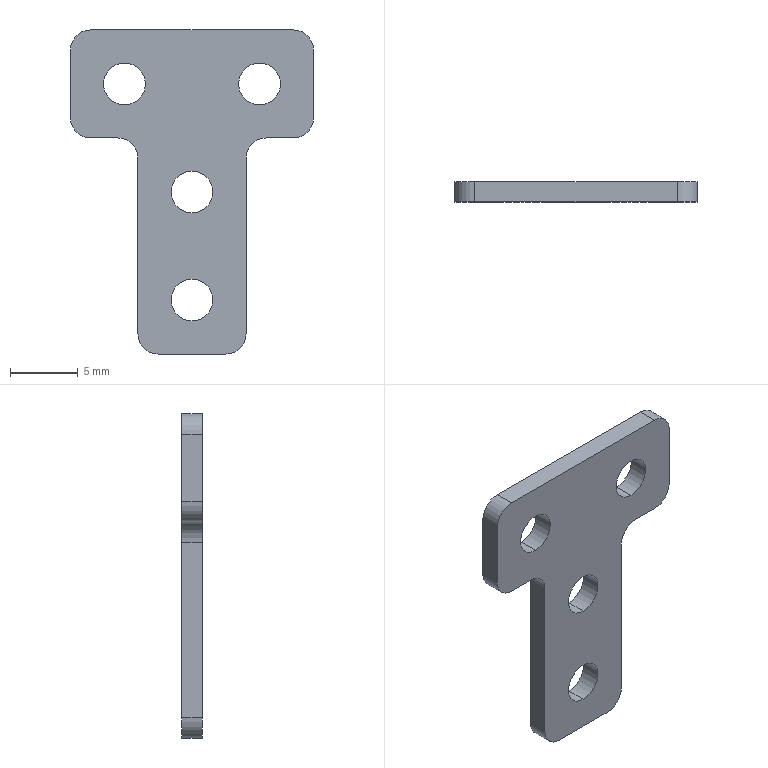Part | SolidWorks | features Extrusion 1, Fillet 1 | 1 solid | 26 faces | box 18 x 1.5 x 24 mm | volume 359.817 mm3 | cylinder 16 | plane 10 | commonest cylinder face diameters 3 x8 3.1 x8
STEP:
#1=CARTESIAN_POINT('',(-5.,1.5,-1.55));
#2=VERTEX_POINT('',#1);
#3=CARTESIAN_POINT('',(-5.,1.5,1.55));
#4=VERTEX_POINT('',#3);
#5=CARTESIAN_POINT('',(-5.,1.5,0.));
#6=DIRECTION('',(0.,1.,0.));
#7=DIRECTION('',(0.,0.,-1.));
#8=AXIS2_PLACEMENT_3D('',#5,#6,#7);
#9=CIRCLE('',#8,1.55);
#10=EDGE_CURVE('',#2,#4,#9,.T.);
#11=ORIENTED_EDGE('',*,*,#10,.T.);
#12=CARTESIAN_POINT('',(-5.,0.,1.55));
#13=VERTEX_POINT('',#12);
#14=CARTESIAN_POINT('',(-5.,1.5,1.55));
#15=DIRECTION('',(0.,-1.,0.));
#16=VECTOR('',#15,1000.);
#17=LINE('',#14,#16);
#18=EDGE_CURVE('',#4,#13,#17,.T.);
#19=ORIENTED_EDGE('',*,*,#18,.T.);
#20=CARTESIAN_POINT('',(-5.,0.,-1.55));
#21=VERTEX_POINT('',#20);
#22=CARTESIAN_POINT('',(-5.,0.,0.));
#23=DIRECTION('',(0.,1.,0.));
#24=DIRECTION('',(0.,0.,-1.));
#25=AXIS2_PLACEMENT_3D('',#22,#23,#24);
#26=CIRCLE('',#25,1.55);
#27=EDGE_CURVE('',#21,#13,#26,.T.);
#28=ORIENTED_EDGE('',*,*,#27,.F.);
#29=CARTESIAN_POINT('',(-5.,1.5,-1.55));
#30=DIRECTION('',(0.,-1.,0.));
#31=VECTOR('',#30,1000.);
#32=LINE('',#29,#31);
#33=EDGE_CURVE('',#2,#21,#32,.T.);
#34=ORIENTED_EDGE('',*,*,#33,.F.);
#35=EDGE_LOOP('',(#11,#19,#28,#34));
#36=FACE_OUTER_BOUND('',#35,.T.);
#37=CARTESIAN_POINT('',(-5.,1.5,0.));
#38=DIRECTION('',(0.,-1.,0.));
#39=DIRECTION('',(0.,0.,-1.));
#40=AXIS2_PLACEMENT_3D('',#37,#38,#39);
#41=CYLINDRICAL_SURFACE('',#40,1.55);
#42=ADVANCED_FACE('',(#36),#41,.F.);
#43=CARTESIAN_POINT('',(0.,1.5,-17.55));
#44=VERTEX_POINT('',#43);
#45=CARTESIAN_POINT('',(0.,1.5,-14.45));
#46=VERTEX_POINT('',#45);
#47=CARTESIAN_POINT('',(0.,1.5,-16.));
#48=DIRECTION('',(0.,1.,0.));
#49=DIRECTION('',(0.,0.,1.));
#50=AXIS2_PLACEMENT_3D('',#47,#48,#49);
#51=CIRCLE('',#50,1.55);
#52=EDGE_CURVE('',#44,#46,#51,.T.);
#53=ORIENTED_EDGE('',*,*,#52,.T.);
#54=CARTESIAN_POINT('',(0.,0.,-14.45));
#55=VERTEX_POINT('',#54);
#56=CARTESIAN_POINT('',(0.,1.5,-14.45));
#57=DIRECTION('',(0.,-1.,0.));
#58=VECTOR('',#57,1000.);
#59=LINE('',#56,#58);
#60=EDGE_CURVE('',#46,#55,#59,.T.);
#61=ORIENTED_EDGE('',*,*,#60,.T.);
#62=CARTESIAN_POINT('',(0.,0.,-17.55));
#63=VERTEX_POINT('',#62);
#64=CARTESIAN_POINT('',(0.,0.,-16.));
#65=DIRECTION('',(0.,1.,0.));
#66=DIRECTION('',(0.,0.,1.));
#67=AXIS2_PLACEMENT_3D('',#64,#65,#66);
#68=CIRCLE('',#67,1.55);
#69=EDGE_CURVE('',#63,#55,#68,.T.);
#70=ORIENTED_EDGE('',*,*,#69,.F.);
#71=CARTESIAN_POINT('',(0.,1.5,-17.55));
#72=DIRECTION('',(0.,-1.,0.));
#73=VECTOR('',#72,1000.);
#74=LINE('',#71,#73);
#75=EDGE_CURVE('',#44,#63,#74,.T.);
#76=ORIENTED_EDGE('',*,*,#75,.F.);
#77=EDGE_LOOP('',(#53,#61,#70,#76));
#78=FACE_OUTER_BOUND('',#77,.T.);
#79=CARTESIAN_POINT('',(0.,1.5,-16.));
#80=DIRECTION('',(0.,-1.,0.));
#81=DIRECTION('',(0.,0.,-1.));
#82=AXIS2_PLACEMENT_3D('',#79,#80,#81);
#83=CYLINDRICAL_SURFACE('',#82,1.55);
#84=ADVANCED_FACE('',(#78),#83,.F.);
#85=CARTESIAN_POINT('',(0.,1.5,-9.55));
#86=VERTEX_POINT('',#85);
#87=CARTESIAN_POINT('',(0.,1.5,-6.45));
#88=VERTEX_POINT('',#87);
#89=CARTESIAN_POINT('',(0.,1.5,-8.));
#90=DIRECTION('',(0.,1.,0.));
#91=DIRECTION('',(0.,0.,1.));
#92=AXIS2_PLACEMENT_3D('',#89,#90,#91);
#93=CIRCLE('',#92,1.55);
#94=EDGE_CURVE('',#86,#88,#93,.T.);
#95=ORIENTED_EDGE('',*,*,#94,.T.);
#96=CARTESIAN_POINT('',(0.,0.,-6.45));
#97=VERTEX_POINT('',#96);
#98=CARTESIAN_POINT('',(0.,1.5,-6.45));
#99=DIRECTION('',(0.,-1.,0.));
#100=VECTOR('',#99,1000.);
#101=LINE('',#98,#100);
#102=EDGE_CURVE('',#88,#97,#101,.T.);
#103=ORIENTED_EDGE('',*,*,#102,.T.);
#104=CARTESIAN_POINT('',(0.,0.,-9.55));
#105=VERTEX_POINT('',#104);
#106=CARTESIAN_POINT('',(0.,0.,-8.));
#107=DIRECTION('',(0.,1.,0.));
#108=DIRECTION('',(0.,0.,1.));
#109=AXIS2_PLACEMENT_3D('',#106,#107,#108);
#110=CIRCLE('',#109,1.55);
#111=EDGE_CURVE('',#105,#97,#110,.T.);
#112=ORIENTED_EDGE('',*,*,#111,.F.);
#113=CARTESIAN_POINT('',(0.,1.5,-9.55));
#114=DIRECTION('',(0.,-1.,0.));
#115=VECTOR('',#114,1000.);
#116=LINE('',#113,#115);
#117=EDGE_CURVE('',#86,#105,#116,.T.);
#118=ORIENTED_EDGE('',*,*,#117,.F.);
#119=EDGE_LOOP('',(#95,#103,#112,#118));
#120=FACE_OUTER_BOUND('',#119,.T.);
#121=CARTESIAN_POINT('',(0.,1.5,-8.));
#122=DIRECTION('',(0.,-1.,0.));
#123=DIRECTION('',(0.,0.,-1.));
#124=AXIS2_PLACEMENT_3D('',#121,#122,#123);
#125=CYLINDRICAL_SURFACE('',#124,1.55);
#126=ADVANCED_FACE('',(#120),#125,.F.);
#127=CARTESIAN_POINT('',(5.,1.5,-1.55));
#128=VERTEX_POINT('',#127);
#129=CARTESIAN_POINT('',(5.,1.5,1.55));
#130=VERTEX_POINT('',#129);
#131=CARTESIAN_POINT('',(5.,1.5,0.));
#132=DIRECTION('',(0.,1.,0.));
#133=DIRECTION('',(0.,0.,1.));
#134=AXIS2_PLACEMENT_3D('',#131,#132,#133);
#135=CIRCLE('',#134,1.55);
#136=EDGE_CURVE('',#128,#130,#135,.T.);
#137=ORIENTED_EDGE('',*,*,#136,.T.);
#138=CARTESIAN_POINT('',(5.,0.,1.55));
#139=VERTEX_POINT('',#138);
#140=CARTESIAN_POINT('',(5.,1.5,1.55));
#141=DIRECTION('',(0.,-1.,0.));
#142=VECTOR('',#141,1000.);
#143=LINE('',#140,#142);
#144=EDGE_CURVE('',#130,#139,#143,.T.);
#145=ORIENTED_EDGE('',*,*,#144,.T.);
#146=CARTESIAN_POINT('',(5.,0.,-1.55));
#147=VERTEX_POINT('',#146);
#148=CARTESIAN_POINT('',(5.,0.,0.));
#149=DIRECTION('',(0.,1.,0.));
#150=DIRECTION('',(0.,0.,1.));
#151=AXIS2_PLACEMENT_3D('',#148,#149,#150);
#152=CIRCLE('',#151,1.55);
#153=EDGE_CURVE('',#147,#139,#152,.T.);
#154=ORIENTED_EDGE('',*,*,#153,.F.);
#155=CARTESIAN_POINT('',(5.,1.5,-1.55));
#156=DIRECTION('',(0.,-1.,0.));
#157=VECTOR('',#156,1000.);
#158=LINE('',#155,#157);
#159=EDGE_CURVE('',#128,#147,#158,.T.);
#160=ORIENTED_EDGE('',*,*,#159,.F.);
#161=EDGE_LOOP('',(#137,#145,#154,#160));
#162=FACE_OUTER_BOUND('',#161,.T.);
#163=CARTESIAN_POINT('',(5.,1.5,0.));
#164=DIRECTION('',(0.,-1.,0.));
#165=DIRECTION('',(0.,0.,-1.));
#166=AXIS2_PLACEMENT_3D('',#163,#164,#165);
#167=CYLINDRICAL_SURFACE('',#166,1.55);
#168=ADVANCED_FACE('',(#162),#167,.F.);
#169=ORIENTED_EDGE('',*,*,#52,.F.);
#170=CARTESIAN_POINT('',(0.,1.5,-16.));
#171=DIRECTION('',(0.,1.,0.));
#172=DIRECTION('',(0.,0.,1.));
#173=AXIS2_PLACEMENT_3D('',#170,#171,#172);
#174=CIRCLE('',#173,1.55);
#175=EDGE_CURVE('',#46,#44,#174,.T.);
#176=ORIENTED_EDGE('',*,*,#175,.F.);
#177=EDGE_LOOP('',(#169,#176));
#178=FACE_BOUND('',#177,.T.);
#179=ORIENTED_EDGE('',*,*,#136,.F.);
#180=CARTESIAN_POINT('',(5.,1.5,0.));
#181=DIRECTION('',(0.,1.,0.));
#182=DIRECTION('',(0.,0.,1.));
#183=AXIS2_PLACEMENT_3D('',#180,#181,#182);
#184=CIRCLE('',#183,1.55);
#185=EDGE_CURVE('',#130,#128,#184,.T.);
#186=ORIENTED_EDGE('',*,*,#185,.F.);
#187=EDGE_LOOP('',(#179,#186));
#188=FACE_BOUND('',#187,.T.);
#189=CARTESIAN_POINT('',(9.,1.5,2.5));
#190=VERTEX_POINT('',#189);
#191=CARTESIAN_POINT('',(9.,1.5,-2.5));
#192=VERTEX_POINT('',#191);
#193=CARTESIAN_POINT('',(9.,1.5,-4.));
#194=DIRECTION('',(0.,0.,-1.));
#195=VECTOR('',#194,1000.);
#196=LINE('',#193,#195);
#197=EDGE_CURVE('',#190,#192,#196,.T.);
#198=ORIENTED_EDGE('',*,*,#197,.T.);
#199=CARTESIAN_POINT('',(7.5,1.5,-4.));
#200=VERTEX_POINT('',#199);
#201=CARTESIAN_POINT('',(7.5,1.5,-2.5));
#202=DIRECTION('',(0.,1.,0.));
#203=DIRECTION('',(0.,0.,1.));
#204=AXIS2_PLACEMENT_3D('',#201,#202,#203);
#205=CIRCLE('',#204,1.5);
#206=EDGE_CURVE('',#192,#200,#205,.T.);
#207=ORIENTED_EDGE('',*,*,#206,.T.);
#208=CARTESIAN_POINT('',(5.5,1.5,-4.));
#209=VERTEX_POINT('',#208);
#210=CARTESIAN_POINT('',(4.,1.5,-4.));
#211=DIRECTION('',(-1.,0.,0.));
#212=VECTOR('',#211,1000.);
#213=LINE('',#210,#212);
#214=EDGE_CURVE('',#200,#209,#213,.T.);
#215=ORIENTED_EDGE('',*,*,#214,.T.);
#216=CARTESIAN_POINT('',(4.,1.5,-5.5));
#217=VERTEX_POINT('',#216);
#218=CARTESIAN_POINT('',(5.5,1.5,-5.5));
#219=DIRECTION('',(0.,-1.,0.));
#220=DIRECTION('',(0.,0.,1.));
#221=AXIS2_PLACEMENT_3D('',#218,#219,#220);
#222=CIRCLE('',#221,1.5);
#223=EDGE_CURVE('',#209,#217,#222,.T.);
#224=ORIENTED_EDGE('',*,*,#223,.T.);
#225=CARTESIAN_POINT('',(4.,1.5,-18.5));
#226=VERTEX_POINT('',#225);
#227=CARTESIAN_POINT('',(4.,1.5,-20.));
#228=DIRECTION('',(0.,0.,-1.));
#229=VECTOR('',#228,1000.);
#230=LINE('',#227,#229);
#231=EDGE_CURVE('',#217,#226,#230,.T.);
#232=ORIENTED_EDGE('',*,*,#231,.T.);
#233=CARTESIAN_POINT('',(2.5,1.5,-20.));
#234=VERTEX_POINT('',#233);
#235=CARTESIAN_POINT('',(2.5,1.5,-18.5));
#236=DIRECTION('',(0.,1.,0.));
#237=DIRECTION('',(0.,0.,1.));
#238=AXIS2_PLACEMENT_3D('',#235,#236,#237);
#239=CIRCLE('',#238,1.5);
#240=EDGE_CURVE('',#226,#234,#239,.T.);
#241=ORIENTED_EDGE('',*,*,#240,.T.);
#242=CARTESIAN_POINT('',(-2.5,1.5,-20.));
#243=VERTEX_POINT('',#242);
#244=CARTESIAN_POINT('',(-4.,1.5,-20.));
#245=DIRECTION('',(-1.,0.,0.));
#246=VECTOR('',#245,1000.);
#247=LINE('',#244,#246);
#248=EDGE_CURVE('',#234,#243,#247,.T.);
#249=ORIENTED_EDGE('',*,*,#248,.T.);
#250=CARTESIAN_POINT('',(-4.,1.5,-18.5));
#251=VERTEX_POINT('',#250);
#252=CARTESIAN_POINT('',(-2.5,1.5,-18.5));
#253=DIRECTION('',(0.,1.,0.));
#254=DIRECTION('',(0.,0.,1.));
#255=AXIS2_PLACEMENT_3D('',#252,#253,#254);
#256=CIRCLE('',#255,1.5);
#257=EDGE_CURVE('',#243,#251,#256,.T.);
#258=ORIENTED_EDGE('',*,*,#257,.T.);
#259=CARTESIAN_POINT('',(-4.,1.5,-5.5));
#260=VERTEX_POINT('',#259);
#261=CARTESIAN_POINT('',(-4.,1.5,-20.));
#262=DIRECTION('',(0.,0.,1.));
#263=VECTOR('',#262,1000.);
#264=LINE('',#261,#263);
#265=EDGE_CURVE('',#251,#260,#264,.T.);
#266=ORIENTED_EDGE('',*,*,#265,.T.);
#267=CARTESIAN_POINT('',(-5.5,1.5,-4.));
#268=VERTEX_POINT('',#267);
#269=CARTESIAN_POINT('',(-5.5,1.5,-5.5));
#270=DIRECTION('',(0.,-1.,0.));
#271=DIRECTION('',(0.,0.,1.));
#272=AXIS2_PLACEMENT_3D('',#269,#270,#271);
#273=CIRCLE('',#272,1.5);
#274=EDGE_CURVE('',#260,#268,#273,.T.);
#275=ORIENTED_EDGE('',*,*,#274,.T.);
#276=CARTESIAN_POINT('',(-7.5,1.5,-4.));
#277=VERTEX_POINT('',#276);
#278=CARTESIAN_POINT('',(-4.,1.5,-4.));
#279=DIRECTION('',(-1.,0.,0.));
#280=VECTOR('',#279,1000.);
#281=LINE('',#278,#280);
#282=EDGE_CURVE('',#268,#277,#281,.T.);
#283=ORIENTED_EDGE('',*,*,#282,.T.);
#284=CARTESIAN_POINT('',(-9.,1.5,-2.5));
#285=VERTEX_POINT('',#284);
#286=CARTESIAN_POINT('',(-7.5,1.5,-2.5));
#287=DIRECTION('',(0.,1.,0.));
#288=DIRECTION('',(0.,0.,1.));
#289=AXIS2_PLACEMENT_3D('',#286,#287,#288);
#290=CIRCLE('',#289,1.5);
#291=EDGE_CURVE('',#277,#285,#290,.T.);
#292=ORIENTED_EDGE('',*,*,#291,.T.);
#293=CARTESIAN_POINT('',(-9.,1.5,2.5));
#294=VERTEX_POINT('',#293);
#295=CARTESIAN_POINT('',(-9.,1.5,-4.));
#296=DIRECTION('',(0.,0.,1.));
#297=VECTOR('',#296,1000.);
#298=LINE('',#295,#297);
#299=EDGE_CURVE('',#285,#294,#298,.T.);
#300=ORIENTED_EDGE('',*,*,#299,.T.);
#301=CARTESIAN_POINT('',(-7.5,1.5,4.));
#302=VERTEX_POINT('',#301);
#303=CARTESIAN_POINT('',(-7.5,1.5,2.5));
#304=DIRECTION('',(0.,1.,0.));
#305=DIRECTION('',(0.,0.,1.));
#306=AXIS2_PLACEMENT_3D('',#303,#304,#305);
#307=CIRCLE('',#306,1.5);
#308=EDGE_CURVE('',#294,#302,#307,.T.);
#309=ORIENTED_EDGE('',*,*,#308,.T.);
#310=CARTESIAN_POINT('',(7.5,1.5,4.));
#311=VERTEX_POINT('',#310);
#312=CARTESIAN_POINT('',(9.,1.5,4.));
#313=DIRECTION('',(1.,0.,0.));
#314=VECTOR('',#313,1000.);
#315=LINE('',#312,#314);
#316=EDGE_CURVE('',#302,#311,#315,.T.);
#317=ORIENTED_EDGE('',*,*,#316,.T.);
#318=CARTESIAN_POINT('',(7.5,1.5,2.5));
#319=DIRECTION('',(0.,1.,0.));
#320=DIRECTION('',(0.,0.,1.));
#321=AXIS2_PLACEMENT_3D('',#318,#319,#320);
#322=CIRCLE('',#321,1.5);
#323=EDGE_CURVE('',#311,#190,#322,.T.);
#324=ORIENTED_EDGE('',*,*,#323,.T.);
#325=EDGE_LOOP('',(#198,#207,#215,#224,#232,#241,#249,#258,#266,#275,#283,#292,#300,#309,#317,#324));
#326=FACE_OUTER_BOUND('',#325,.T.);
#327=ORIENTED_EDGE('',*,*,#94,.F.);
#328=CARTESIAN_POINT('',(0.,1.5,-8.));
#329=DIRECTION('',(0.,1.,0.));
#330=DIRECTION('',(0.,0.,1.));
#331=AXIS2_PLACEMENT_3D('',#328,#329,#330);
#332=CIRCLE('',#331,1.55);
#333=EDGE_CURVE('',#88,#86,#332,.T.);
#334=ORIENTED_EDGE('',*,*,#333,.F.);
#335=EDGE_LOOP('',(#327,#334));
#336=FACE_BOUND('',#335,.T.);
#337=ORIENTED_EDGE('',*,*,#10,.F.);
#338=CARTESIAN_POINT('',(-5.,1.5,0.));
#339=DIRECTION('',(0.,1.,0.));
#340=DIRECTION('',(0.,0.,-1.));
#341=AXIS2_PLACEMENT_3D('',#338,#339,#340);
#342=CIRCLE('',#341,1.55);
#343=EDGE_CURVE('',#4,#2,#342,.T.);
#344=ORIENTED_EDGE('',*,*,#343,.F.);
#345=EDGE_LOOP('',(#337,#344));
#346=FACE_BOUND('',#345,.T.);
#347=CARTESIAN_POINT('',(0.,1.5,0.));
#348=DIRECTION('',(0.,1.,0.));
#349=DIRECTION('',(0.,0.,1.));
#350=AXIS2_PLACEMENT_3D('',#347,#348,#349);
#351=PLANE('',#350);
#352=ADVANCED_FACE('',(#178,#188,#326,#336,#346),#351,.T.);
#353=CARTESIAN_POINT('',(7.5,0.,-4.));
#354=VERTEX_POINT('',#353);
#355=CARTESIAN_POINT('',(5.5,0.,-4.));
#356=VERTEX_POINT('',#355);
#357=CARTESIAN_POINT('',(4.,0.,-4.));
#358=DIRECTION('',(-1.,0.,0.));
#359=VECTOR('',#358,1000.);
#360=LINE('',#357,#359);
#361=EDGE_CURVE('',#354,#356,#360,.T.);
#362=ORIENTED_EDGE('',*,*,#361,.F.);
#363=CARTESIAN_POINT('',(9.,0.,-2.5));
#364=VERTEX_POINT('',#363);
#365=CARTESIAN_POINT('',(7.5,0.,-2.5));
#366=DIRECTION('',(0.,-1.,0.));
#367=DIRECTION('',(0.,0.,1.));
#368=AXIS2_PLACEMENT_3D('',#365,#366,#367);
#369=CIRCLE('',#368,1.5);
#370=EDGE_CURVE('',#354,#364,#369,.T.);
#371=ORIENTED_EDGE('',*,*,#370,.T.);
#372=CARTESIAN_POINT('',(9.,0.,2.5));
#373=VERTEX_POINT('',#372);
#374=CARTESIAN_POINT('',(9.,0.,-4.));
#375=DIRECTION('',(0.,0.,-1.));
#376=VECTOR('',#375,1000.);
#377=LINE('',#374,#376);
#378=EDGE_CURVE('',#373,#364,#377,.T.);
#379=ORIENTED_EDGE('',*,*,#378,.F.);
#380=CARTESIAN_POINT('',(7.5,0.,4.));
#381=VERTEX_POINT('',#380);
#382=CARTESIAN_POINT('',(7.5,0.,2.5));
#383=DIRECTION('',(0.,-1.,0.));
#384=DIRECTION('',(0.,0.,1.));
#385=AXIS2_PLACEMENT_3D('',#382,#383,#384);
#386=CIRCLE('',#385,1.5);
#387=EDGE_CURVE('',#373,#381,#386,.T.);
#388=ORIENTED_EDGE('',*,*,#387,.T.);
#389=CARTESIAN_POINT('',(-7.5,0.,4.));
#390=VERTEX_POINT('',#389);
#391=CARTESIAN_POINT('',(9.,0.,4.));
#392=DIRECTION('',(1.,0.,0.));
#393=VECTOR('',#392,1000.);
#394=LINE('',#391,#393);
#395=EDGE_CURVE('',#390,#381,#394,.T.);
#396=ORIENTED_EDGE('',*,*,#395,.F.);
#397=CARTESIAN_POINT('',(-9.,0.,2.5));
#398=VERTEX_POINT('',#397);
#399=CARTESIAN_POINT('',(-7.5,0.,2.5));
#400=DIRECTION('',(0.,-1.,0.));
#401=DIRECTION('',(0.,0.,1.));
#402=AXIS2_PLACEMENT_3D('',#399,#400,#401);
#403=CIRCLE('',#402,1.5);
#404=EDGE_CURVE('',#390,#398,#403,.T.);
#405=ORIENTED_EDGE('',*,*,#404,.T.);
#406=CARTESIAN_POINT('',(-9.,0.,-2.5));
#407=VERTEX_POINT('',#406);
#408=CARTESIAN_POINT('',(-9.,0.,-4.));
#409=DIRECTION('',(0.,0.,1.));
#410=VECTOR('',#409,1000.);
#411=LINE('',#408,#410);
#412=EDGE_CURVE('',#407,#398,#411,.T.);
#413=ORIENTED_EDGE('',*,*,#412,.F.);
#414=CARTESIAN_POINT('',(-7.5,0.,-4.));
#415=VERTEX_POINT('',#414);
#416=CARTESIAN_POINT('',(-7.5,0.,-2.5));
#417=DIRECTION('',(0.,-1.,0.));
#418=DIRECTION('',(0.,0.,1.));
#419=AXIS2_PLACEMENT_3D('',#416,#417,#418);
#420=CIRCLE('',#419,1.5);
#421=EDGE_CURVE('',#407,#415,#420,.T.);
#422=ORIENTED_EDGE('',*,*,#421,.T.);
#423=CARTESIAN_POINT('',(-5.5,0.,-4.));
#424=VERTEX_POINT('',#423);
#425=CARTESIAN_POINT('',(-4.,0.,-4.));
#426=DIRECTION('',(-1.,0.,0.));
#427=VECTOR('',#426,1000.);
#428=LINE('',#425,#427);
#429=EDGE_CURVE('',#424,#415,#428,.T.);
#430=ORIENTED_EDGE('',*,*,#429,.F.);
#431=CARTESIAN_POINT('',(-4.,0.,-5.5));
#432=VERTEX_POINT('',#431);
#433=CARTESIAN_POINT('',(-5.5,0.,-5.5));
#434=DIRECTION('',(0.,1.,0.));
#435=DIRECTION('',(0.,0.,1.));
#436=AXIS2_PLACEMENT_3D('',#433,#434,#435);
#437=CIRCLE('',#436,1.5);
#438=EDGE_CURVE('',#424,#432,#437,.T.);
#439=ORIENTED_EDGE('',*,*,#438,.T.);
#440=CARTESIAN_POINT('',(-4.,0.,-18.5));
#441=VERTEX_POINT('',#440);
#442=CARTESIAN_POINT('',(-4.,0.,-20.));
#443=DIRECTION('',(0.,0.,1.));
#444=VECTOR('',#443,1000.);
#445=LINE('',#442,#444);
#446=EDGE_CURVE('',#441,#432,#445,.T.);
#447=ORIENTED_EDGE('',*,*,#446,.F.);
#448=CARTESIAN_POINT('',(-2.5,0.,-20.));
#449=VERTEX_POINT('',#448);
#450=CARTESIAN_POINT('',(-2.5,0.,-18.5));
#451=DIRECTION('',(0.,-1.,0.));
#452=DIRECTION('',(0.,0.,1.));
#453=AXIS2_PLACEMENT_3D('',#450,#451,#452);
#454=CIRCLE('',#453,1.5);
#455=EDGE_CURVE('',#441,#449,#454,.T.);
#456=ORIENTED_EDGE('',*,*,#455,.T.);
#457=CARTESIAN_POINT('',(2.5,0.,-20.));
#458=VERTEX_POINT('',#457);
#459=CARTESIAN_POINT('',(-4.,0.,-20.));
#460=DIRECTION('',(-1.,0.,0.));
#461=VECTOR('',#460,1000.);
#462=LINE('',#459,#461);
#463=EDGE_CURVE('',#458,#449,#462,.T.);
#464=ORIENTED_EDGE('',*,*,#463,.F.);
#465=CARTESIAN_POINT('',(4.,0.,-18.5));
#466=VERTEX_POINT('',#465);
#467=CARTESIAN_POINT('',(2.5,0.,-18.5));
#468=DIRECTION('',(0.,-1.,0.));
#469=DIRECTION('',(0.,0.,1.));
#470=AXIS2_PLACEMENT_3D('',#467,#468,#469);
#471=CIRCLE('',#470,1.5);
#472=EDGE_CURVE('',#458,#466,#471,.T.);
#473=ORIENTED_EDGE('',*,*,#472,.T.);
#474=CARTESIAN_POINT('',(4.,0.,-5.5));
#475=VERTEX_POINT('',#474);
#476=CARTESIAN_POINT('',(4.,0.,-20.));
#477=DIRECTION('',(0.,0.,-1.));
#478=VECTOR('',#477,1000.);
#479=LINE('',#476,#478);
#480=EDGE_CURVE('',#475,#466,#479,.T.);
#481=ORIENTED_EDGE('',*,*,#480,.F.);
#482=CARTESIAN_POINT('',(5.5,0.,-5.5));
#483=DIRECTION('',(0.,1.,0.));
#484=DIRECTION('',(0.,0.,1.));
#485=AXIS2_PLACEMENT_3D('',#482,#483,#484);
#486=CIRCLE('',#485,1.5);
#487=EDGE_CURVE('',#475,#356,#486,.T.);
#488=ORIENTED_EDGE('',*,*,#487,.T.);
#489=EDGE_LOOP('',(#362,#371,#379,#388,#396,#405,#413,#422,#430,#439,#447,#456,#464,#473,#481,#488));
#490=FACE_OUTER_BOUND('',#489,.T.);
#491=ORIENTED_EDGE('',*,*,#153,.T.);
#492=CARTESIAN_POINT('',(5.,0.,0.));
#493=DIRECTION('',(0.,1.,0.));
#494=DIRECTION('',(0.,0.,1.));
#495=AXIS2_PLACEMENT_3D('',#492,#493,#494);
#496=CIRCLE('',#495,1.55);
#497=EDGE_CURVE('',#139,#147,#496,.T.);
#498=ORIENTED_EDGE('',*,*,#497,.T.);
#499=EDGE_LOOP('',(#491,#498));
#500=FACE_BOUND('',#499,.T.);
#501=ORIENTED_EDGE('',*,*,#111,.T.);
#502=CARTESIAN_POINT('',(0.,0.,-8.));
#503=DIRECTION('',(0.,1.,0.));
#504=DIRECTION('',(0.,0.,1.));
#505=AXIS2_PLACEMENT_3D('',#502,#503,#504);
#506=CIRCLE('',#505,1.55);
#507=EDGE_CURVE('',#97,#105,#506,.T.);
#508=ORIENTED_EDGE('',*,*,#507,.T.);
#509=EDGE_LOOP('',(#501,#508));
#510=FACE_BOUND('',#509,.T.);
#511=ORIENTED_EDGE('',*,*,#69,.T.);
#512=CARTESIAN_POINT('',(0.,0.,-16.));
#513=DIRECTION('',(0.,1.,0.));
#514=DIRECTION('',(0.,0.,1.));
#515=AXIS2_PLACEMENT_3D('',#512,#513,#514);
#516=CIRCLE('',#515,1.55);
#517=EDGE_CURVE('',#55,#63,#516,.T.);
#518=ORIENTED_EDGE('',*,*,#517,.T.);
#519=EDGE_LOOP('',(#511,#518));
#520=FACE_BOUND('',#519,.T.);
#521=ORIENTED_EDGE('',*,*,#27,.T.);
#522=CARTESIAN_POINT('',(-5.,0.,0.));
#523=DIRECTION('',(0.,1.,0.));
#524=DIRECTION('',(0.,0.,-1.));
#525=AXIS2_PLACEMENT_3D('',#522,#523,#524);
#526=CIRCLE('',#525,1.55);
#527=EDGE_CURVE('',#13,#21,#526,.T.);
#528=ORIENTED_EDGE('',*,*,#527,.T.);
#529=EDGE_LOOP('',(#521,#528));
#530=FACE_BOUND('',#529,.T.);
#531=CARTESIAN_POINT('',(0.,0.,0.));
#532=DIRECTION('',(0.,1.,0.));
#533=DIRECTION('',(0.,0.,1.));
#534=AXIS2_PLACEMENT_3D('',#531,#532,#533);
#535=PLANE('',#534);
#536=ADVANCED_FACE('',(#490,#500,#510,#520,#530),#535,.F.);
#537=ORIENTED_EDGE('',*,*,#231,.F.);
#538=CARTESIAN_POINT('',(4.,0.,-5.5));
#539=DIRECTION('',(0.,-1.,0.));
#540=VECTOR('',#539,1000.);
#541=LINE('',#538,#540);
#542=EDGE_CURVE('',#217,#475,#541,.T.);
#543=ORIENTED_EDGE('',*,*,#542,.T.);
#544=ORIENTED_EDGE('',*,*,#480,.T.);
#545=CARTESIAN_POINT('',(4.,1.5,-18.5));
#546=DIRECTION('',(0.,1.,0.));
#547=VECTOR('',#546,1000.);
#548=LINE('',#545,#547);
#549=EDGE_CURVE('',#466,#226,#548,.T.);
#550=ORIENTED_EDGE('',*,*,#549,.T.);
#551=EDGE_LOOP('',(#537,#543,#544,#550));
#552=FACE_OUTER_BOUND('',#551,.T.);
#553=CARTESIAN_POINT('',(4.,1.5,-20.));
#554=DIRECTION('',(-1.,0.,0.));
#555=DIRECTION('',(0.,0.,1.));
#556=AXIS2_PLACEMENT_3D('',#553,#554,#555);
#557=PLANE('',#556);
#558=ADVANCED_FACE('',(#552),#557,.F.);
#559=ORIENTED_EDGE('',*,*,#463,.T.);
#560=CARTESIAN_POINT('',(-2.5,1.5,-20.));
#561=DIRECTION('',(0.,1.,0.));
#562=VECTOR('',#561,1000.);
#563=LINE('',#560,#562);
#564=EDGE_CURVE('',#449,#243,#563,.T.);
#565=ORIENTED_EDGE('',*,*,#564,.T.);
#566=ORIENTED_EDGE('',*,*,#248,.F.);
#567=CARTESIAN_POINT('',(2.5,1.5,-20.));
#568=DIRECTION('',(0.,-1.,0.));
#569=VECTOR('',#568,1000.);
#570=LINE('',#567,#569);
#571=EDGE_CURVE('',#234,#458,#570,.T.);
#572=ORIENTED_EDGE('',*,*,#571,.T.);
#573=EDGE_LOOP('',(#559,#565,#566,#572));
#574=FACE_OUTER_BOUND('',#573,.T.);
#575=CARTESIAN_POINT('',(-4.,1.5,-20.));
#576=DIRECTION('',(0.,0.,1.));
#577=DIRECTION('',(1.,0.,0.));
#578=AXIS2_PLACEMENT_3D('',#575,#576,#577);
#579=PLANE('',#578);
#580=ADVANCED_FACE('',(#574),#579,.F.);
#581=ORIENTED_EDGE('',*,*,#446,.T.);
#582=CARTESIAN_POINT('',(-4.,1.5,-5.5));
#583=DIRECTION('',(0.,1.,0.));
#584=VECTOR('',#583,1000.);
#585=LINE('',#582,#584);
#586=EDGE_CURVE('',#432,#260,#585,.T.);
#587=ORIENTED_EDGE('',*,*,#586,.T.);
#588=ORIENTED_EDGE('',*,*,#265,.F.);
#589=CARTESIAN_POINT('',(-4.,1.5,-18.5));
#590=DIRECTION('',(0.,-1.,0.));
#591=VECTOR('',#590,1000.);
#592=LINE('',#589,#591);
#593=EDGE_CURVE('',#251,#441,#592,.T.);
#594=ORIENTED_EDGE('',*,*,#593,.T.);
#595=EDGE_LOOP('',(#581,#587,#588,#594));
#596=FACE_OUTER_BOUND('',#595,.T.);
#597=CARTESIAN_POINT('',(-4.,1.5,-20.));
#598=DIRECTION('',(1.,0.,0.));
#599=DIRECTION('',(0.,0.,-1.));
#600=AXIS2_PLACEMENT_3D('',#597,#598,#599);
#601=PLANE('',#600);
#602=ADVANCED_FACE('',(#596),#601,.F.);
#603=ORIENTED_EDGE('',*,*,#282,.F.);
#604=CARTESIAN_POINT('',(-5.5,0.,-4.));
#605=DIRECTION('',(0.,-1.,0.));
#606=VECTOR('',#605,1000.);
#607=LINE('',#604,#606);
#608=EDGE_CURVE('',#268,#424,#607,.T.);
#609=ORIENTED_EDGE('',*,*,#608,.T.);
#610=ORIENTED_EDGE('',*,*,#429,.T.);
#611=CARTESIAN_POINT('',(-7.5,1.5,-4.));
#612=DIRECTION('',(0.,1.,0.));
#613=VECTOR('',#612,1000.);
#614=LINE('',#611,#613);
#615=EDGE_CURVE('',#415,#277,#614,.T.);
#616=ORIENTED_EDGE('',*,*,#615,.T.);
#617=EDGE_LOOP('',(#603,#609,#610,#616));
#618=FACE_OUTER_BOUND('',#617,.T.);
#619=CARTESIAN_POINT('',(-4.,1.5,-4.));
#620=DIRECTION('',(0.,0.,1.));
#621=DIRECTION('',(1.,0.,0.));
#622=AXIS2_PLACEMENT_3D('',#619,#620,#621);
#623=PLANE('',#622);
#624=ADVANCED_FACE('',(#618),#623,.F.);
#625=ORIENTED_EDGE('',*,*,#412,.T.);
#626=CARTESIAN_POINT('',(-9.,1.5,2.5));
#627=DIRECTION('',(0.,1.,0.));
#628=VECTOR('',#627,1000.);
#629=LINE('',#626,#628);
#630=EDGE_CURVE('',#398,#294,#629,.T.);
#631=ORIENTED_EDGE('',*,*,#630,.T.);
#632=ORIENTED_EDGE('',*,*,#299,.F.);
#633=CARTESIAN_POINT('',(-9.,1.5,-2.5));
#634=DIRECTION('',(0.,-1.,0.));
#635=VECTOR('',#634,1000.);
#636=LINE('',#633,#635);
#637=EDGE_CURVE('',#285,#407,#636,.T.);
#638=ORIENTED_EDGE('',*,*,#637,.T.);
#639=EDGE_LOOP('',(#625,#631,#632,#638));
#640=FACE_OUTER_BOUND('',#639,.T.);
#641=CARTESIAN_POINT('',(-9.,1.5,-4.));
#642=DIRECTION('',(1.,0.,0.));
#643=DIRECTION('',(0.,0.,-1.));
#644=AXIS2_PLACEMENT_3D('',#641,#642,#643);
#645=PLANE('',#644);
#646=ADVANCED_FACE('',(#640),#645,.F.);
#647=ORIENTED_EDGE('',*,*,#395,.T.);
#648=CARTESIAN_POINT('',(7.5,1.5,4.));
#649=DIRECTION('',(0.,1.,0.));
#650=VECTOR('',#649,1000.);
#651=LINE('',#648,#650);
#652=EDGE_CURVE('',#381,#311,#651,.T.);
#653=ORIENTED_EDGE('',*,*,#652,.T.);
#654=ORIENTED_EDGE('',*,*,#316,.F.);
#655=CARTESIAN_POINT('',(-7.5,1.5,4.));
#656=DIRECTION('',(0.,-1.,0.));
#657=VECTOR('',#656,1000.);
#658=LINE('',#655,#657);
#659=EDGE_CURVE('',#302,#390,#658,.T.);
#660=ORIENTED_EDGE('',*,*,#659,.T.);
#661=EDGE_LOOP('',(#647,#653,#654,#660));
#662=FACE_OUTER_BOUND('',#661,.T.);
#663=CARTESIAN_POINT('',(9.,1.5,4.));
#664=DIRECTION('',(0.,0.,-1.));
#665=DIRECTION('',(-1.,0.,0.));
#666=AXIS2_PLACEMENT_3D('',#663,#664,#665);
#667=PLANE('',#666);
#668=ADVANCED_FACE('',(#662),#667,.F.);
#669=ORIENTED_EDGE('',*,*,#378,.T.);
#670=CARTESIAN_POINT('',(9.,1.5,-2.5));
#671=DIRECTION('',(0.,1.,0.));
#672=VECTOR('',#671,1000.);
#673=LINE('',#670,#672);
#674=EDGE_CURVE('',#364,#192,#673,.T.);
#675=ORIENTED_EDGE('',*,*,#674,.T.);
#676=ORIENTED_EDGE('',*,*,#197,.F.);
#677=CARTESIAN_POINT('',(9.,1.5,2.5));
#678=DIRECTION('',(0.,-1.,0.));
#679=VECTOR('',#678,1000.);
#680=LINE('',#677,#679);
#681=EDGE_CURVE('',#190,#373,#680,.T.);
#682=ORIENTED_EDGE('',*,*,#681,.T.);
#683=EDGE_LOOP('',(#669,#675,#676,#682));
#684=FACE_OUTER_BOUND('',#683,.T.);
#685=CARTESIAN_POINT('',(9.,1.5,-4.));
#686=DIRECTION('',(-1.,0.,0.));
#687=DIRECTION('',(0.,0.,1.));
#688=AXIS2_PLACEMENT_3D('',#685,#686,#687);
#689=PLANE('',#688);
#690=ADVANCED_FACE('',(#684),#689,.F.);
#691=ORIENTED_EDGE('',*,*,#361,.T.);
#692=CARTESIAN_POINT('',(5.5,1.5,-4.));
#693=DIRECTION('',(0.,1.,0.));
#694=VECTOR('',#693,1000.);
#695=LINE('',#692,#694);
#696=EDGE_CURVE('',#356,#209,#695,.T.);
#697=ORIENTED_EDGE('',*,*,#696,.T.);
#698=ORIENTED_EDGE('',*,*,#214,.F.);
#699=CARTESIAN_POINT('',(7.5,1.5,-4.));
#700=DIRECTION('',(0.,-1.,0.));
#701=VECTOR('',#700,1000.);
#702=LINE('',#699,#701);
#703=EDGE_CURVE('',#200,#354,#702,.T.);
#704=ORIENTED_EDGE('',*,*,#703,.T.);
#705=EDGE_LOOP('',(#691,#697,#698,#704));
#706=FACE_OUTER_BOUND('',#705,.T.);
#707=CARTESIAN_POINT('',(4.,1.5,-4.));
#708=DIRECTION('',(0.,0.,1.));
#709=DIRECTION('',(1.,0.,0.));
#710=AXIS2_PLACEMENT_3D('',#707,#708,#709);
#711=PLANE('',#710);
#712=ADVANCED_FACE('',(#706),#711,.F.);
#713=ORIENTED_EDGE('',*,*,#144,.F.);
#714=ORIENTED_EDGE('',*,*,#185,.T.);
#715=ORIENTED_EDGE('',*,*,#159,.T.);
#716=ORIENTED_EDGE('',*,*,#497,.F.);
#717=EDGE_LOOP('',(#713,#714,#715,#716));
#718=FACE_OUTER_BOUND('',#717,.T.);
#719=CARTESIAN_POINT('',(5.,1.5,0.));
#720=DIRECTION('',(0.,-1.,0.));
#721=DIRECTION('',(0.,0.,-1.));
#722=AXIS2_PLACEMENT_3D('',#719,#720,#721);
#723=CYLINDRICAL_SURFACE('',#722,1.55);
#724=ADVANCED_FACE('',(#718),#723,.F.);
#725=ORIENTED_EDGE('',*,*,#102,.F.);
#726=ORIENTED_EDGE('',*,*,#333,.T.);
#727=ORIENTED_EDGE('',*,*,#117,.T.);
#728=ORIENTED_EDGE('',*,*,#507,.F.);
#729=EDGE_LOOP('',(#725,#726,#727,#728));
#730=FACE_OUTER_BOUND('',#729,.T.);
#731=CARTESIAN_POINT('',(0.,1.5,-8.));
#732=DIRECTION('',(0.,-1.,0.));
#733=DIRECTION('',(0.,0.,-1.));
#734=AXIS2_PLACEMENT_3D('',#731,#732,#733);
#735=CYLINDRICAL_SURFACE('',#734,1.55);
#736=ADVANCED_FACE('',(#730),#735,.F.);
#737=ORIENTED_EDGE('',*,*,#60,.F.);
#738=ORIENTED_EDGE('',*,*,#175,.T.);
#739=ORIENTED_EDGE('',*,*,#75,.T.);
#740=ORIENTED_EDGE('',*,*,#517,.F.);
#741=EDGE_LOOP('',(#737,#738,#739,#740));
#742=FACE_OUTER_BOUND('',#741,.T.);
#743=CARTESIAN_POINT('',(0.,1.5,-16.));
#744=DIRECTION('',(0.,-1.,0.));
#745=DIRECTION('',(0.,0.,-1.));
#746=AXIS2_PLACEMENT_3D('',#743,#744,#745);
#747=CYLINDRICAL_SURFACE('',#746,1.55);
#748=ADVANCED_FACE('',(#742),#747,.F.);
#749=ORIENTED_EDGE('',*,*,#18,.F.);
#750=ORIENTED_EDGE('',*,*,#343,.T.);
#751=ORIENTED_EDGE('',*,*,#33,.T.);
#752=ORIENTED_EDGE('',*,*,#527,.F.);
#753=EDGE_LOOP('',(#749,#750,#751,#752));
#754=FACE_OUTER_BOUND('',#753,.T.);
#755=CARTESIAN_POINT('',(-5.,1.5,0.));
#756=DIRECTION('',(0.,-1.,0.));
#757=DIRECTION('',(0.,0.,-1.));
#758=AXIS2_PLACEMENT_3D('',#755,#756,#757);
#759=CYLINDRICAL_SURFACE('',#758,1.55);
#760=ADVANCED_FACE('',(#754),#759,.F.);
#761=ORIENTED_EDGE('',*,*,#223,.F.);
#762=ORIENTED_EDGE('',*,*,#696,.F.);
#763=ORIENTED_EDGE('',*,*,#487,.F.);
#764=ORIENTED_EDGE('',*,*,#542,.F.);
#765=EDGE_LOOP('',(#761,#762,#763,#764));
#766=FACE_OUTER_BOUND('',#765,.T.);
#767=CARTESIAN_POINT('',(5.5,1.5,-5.5));
#768=DIRECTION('',(0.,1.,0.));
#769=DIRECTION('',(0.,0.,1.));
#770=AXIS2_PLACEMENT_3D('',#767,#768,#769);
#771=CYLINDRICAL_SURFACE('',#770,1.5);
#772=ADVANCED_FACE('',(#766),#771,.F.);
#773=ORIENTED_EDGE('',*,*,#206,.F.);
#774=ORIENTED_EDGE('',*,*,#674,.F.);
#775=ORIENTED_EDGE('',*,*,#370,.F.);
#776=ORIENTED_EDGE('',*,*,#703,.F.);
#777=EDGE_LOOP('',(#773,#774,#775,#776));
#778=FACE_OUTER_BOUND('',#777,.T.);
#779=CARTESIAN_POINT('',(7.5,1.5,-2.5));
#780=DIRECTION('',(0.,-1.,0.));
#781=DIRECTION('',(0.,0.,-1.));
#782=AXIS2_PLACEMENT_3D('',#779,#780,#781);
#783=CYLINDRICAL_SURFACE('',#782,1.5);
#784=ADVANCED_FACE('',(#778),#783,.T.);
#785=ORIENTED_EDGE('',*,*,#323,.F.);
#786=ORIENTED_EDGE('',*,*,#652,.F.);
#787=ORIENTED_EDGE('',*,*,#387,.F.);
#788=ORIENTED_EDGE('',*,*,#681,.F.);
#789=EDGE_LOOP('',(#785,#786,#787,#788));
#790=FACE_OUTER_BOUND('',#789,.T.);
#791=CARTESIAN_POINT('',(7.5,1.5,2.5));
#792=DIRECTION('',(0.,-1.,0.));
#793=DIRECTION('',(0.,0.,-1.));
#794=AXIS2_PLACEMENT_3D('',#791,#792,#793);
#795=CYLINDRICAL_SURFACE('',#794,1.5);
#796=ADVANCED_FACE('',(#790),#795,.T.);
#797=ORIENTED_EDGE('',*,*,#274,.F.);
#798=ORIENTED_EDGE('',*,*,#586,.F.);
#799=ORIENTED_EDGE('',*,*,#438,.F.);
#800=ORIENTED_EDGE('',*,*,#608,.F.);
#801=EDGE_LOOP('',(#797,#798,#799,#800));
#802=FACE_OUTER_BOUND('',#801,.T.);
#803=CARTESIAN_POINT('',(-5.5,1.5,-5.5));
#804=DIRECTION('',(0.,1.,0.));
#805=DIRECTION('',(0.,0.,1.));
#806=AXIS2_PLACEMENT_3D('',#803,#804,#805);
#807=CYLINDRICAL_SURFACE('',#806,1.5);
#808=ADVANCED_FACE('',(#802),#807,.F.);
#809=ORIENTED_EDGE('',*,*,#257,.F.);
#810=ORIENTED_EDGE('',*,*,#564,.F.);
#811=ORIENTED_EDGE('',*,*,#455,.F.);
#812=ORIENTED_EDGE('',*,*,#593,.F.);
#813=EDGE_LOOP('',(#809,#810,#811,#812));
#814=FACE_OUTER_BOUND('',#813,.T.);
#815=CARTESIAN_POINT('',(-2.5,1.5,-18.5));
#816=DIRECTION('',(0.,-1.,0.));
#817=DIRECTION('',(0.,0.,-1.));
#818=AXIS2_PLACEMENT_3D('',#815,#816,#817);
#819=CYLINDRICAL_SURFACE('',#818,1.5);
#820=ADVANCED_FACE('',(#814),#819,.T.);
#821=ORIENTED_EDGE('',*,*,#240,.F.);
#822=ORIENTED_EDGE('',*,*,#549,.F.);
#823=ORIENTED_EDGE('',*,*,#472,.F.);
#824=ORIENTED_EDGE('',*,*,#571,.F.);
#825=EDGE_LOOP('',(#821,#822,#823,#824));
#826=FACE_OUTER_BOUND('',#825,.T.);
#827=CARTESIAN_POINT('',(2.5,1.5,-18.5));
#828=DIRECTION('',(0.,-1.,0.));
#829=DIRECTION('',(0.,0.,-1.));
#830=AXIS2_PLACEMENT_3D('',#827,#828,#829);
#831=CYLINDRICAL_SURFACE('',#830,1.5);
#832=ADVANCED_FACE('',(#826),#831,.T.);
#833=ORIENTED_EDGE('',*,*,#308,.F.);
#834=ORIENTED_EDGE('',*,*,#630,.F.);
#835=ORIENTED_EDGE('',*,*,#404,.F.);
#836=ORIENTED_EDGE('',*,*,#659,.F.);
#837=EDGE_LOOP('',(#833,#834,#835,#836));
#838=FACE_OUTER_BOUND('',#837,.T.);
#839=CARTESIAN_POINT('',(-7.5,1.5,2.5));
#840=DIRECTION('',(0.,-1.,0.));
#841=DIRECTION('',(0.,0.,-1.));
#842=AXIS2_PLACEMENT_3D('',#839,#840,#841);
#843=CYLINDRICAL_SURFACE('',#842,1.5);
#844=ADVANCED_FACE('',(#838),#843,.T.);
#845=ORIENTED_EDGE('',*,*,#291,.F.);
#846=ORIENTED_EDGE('',*,*,#615,.F.);
#847=ORIENTED_EDGE('',*,*,#421,.F.);
#848=ORIENTED_EDGE('',*,*,#637,.F.);
#849=EDGE_LOOP('',(#845,#846,#847,#848));
#850=FACE_OUTER_BOUND('',#849,.T.);
#851=CARTESIAN_POINT('',(-7.5,1.5,-2.5));
#852=DIRECTION('',(0.,-1.,0.));
#853=DIRECTION('',(0.,0.,-1.));
#854=AXIS2_PLACEMENT_3D('',#851,#852,#853);
#855=CYLINDRICAL_SURFACE('',#854,1.5);
#856=ADVANCED_FACE('',(#850),#855,.T.);
#857=CLOSED_SHELL('',(#42,#84,#126,#168,#352,#536,#558,#580,#602,#624,#646,#668,#690,#712,#724,#736,#748,#760,#772,#784,#796,#808,#820,#832,#844,#856));
#858=MANIFOLD_SOLID_BREP('',#857);
#859=CARTESIAN_POINT('',(0.,0.,0.));
#860=DIRECTION('',(0.,0.,1.));
#861=DIRECTION('',(1.,0.,0.));
#862=AXIS2_PLACEMENT_3D('',#859,#860,#861);
#863=(LENGTH_UNIT()NAMED_UNIT(*)SI_UNIT(.MILLI.,.METRE.));
#864=UNCERTAINTY_MEASURE_WITH_UNIT(LENGTH_MEASURE(0.00001),#863,'','');
#865=(NAMED_UNIT(*)PLANE_ANGLE_UNIT()SI_UNIT($,.RADIAN.));
#866=(NAMED_UNIT(*)SI_UNIT($,.STERADIAN.)SOLID_ANGLE_UNIT());
#867=(GEOMETRIC_REPRESENTATION_CONTEXT(3)GLOBAL_UNCERTAINTY_ASSIGNED_CONTEXT((#864))GLOBAL_UNIT_ASSIGNED_CONTEXT((#863,#865,#866))REPRESENTATION_CONTEXT('',''));
#868=ADVANCED_BREP_SHAPE_REPRESENTATION('',(#858,#862),#867);